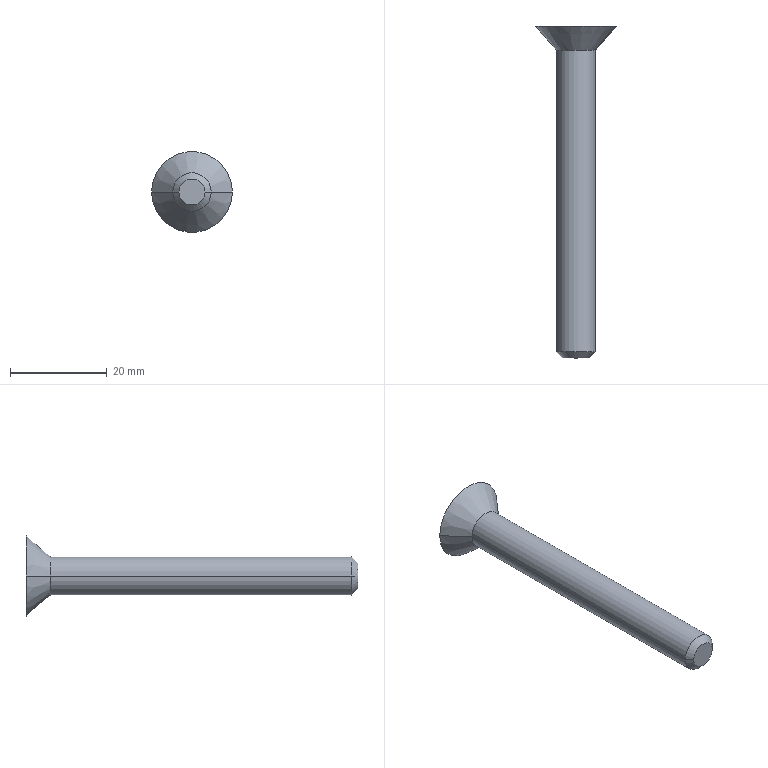Part | NX | features BREP 1 | 1 solid | 15 faces | box 16.681 x 68.529 x 16.681 mm | volume 3731 mm3 | plane 9 | cone 4 | cylinder 2 | commonest cylinder face diameters 7.938 x2
STEP:
#1=CARTESIAN_POINT('',(8.341,0.,0.));
#2=VERTEX_POINT('',#1);
#3=CARTESIAN_POINT('',(3.969,-5.029,0.));
#4=VERTEX_POINT('',#3);
#5=CARTESIAN_POINT('',(3.969,-5.029,0.));
#6=DIRECTION('',(0.6561,0.7547,0.));
#7=VECTOR('',#6,1000.);
#8=LINE('',#5,#7);
#9=EDGE_CURVE('',#2,#4,#8,.F.);
#10=ORIENTED_EDGE('',*,*,#9,.F.);
#11=CARTESIAN_POINT('',(-8.341,0.,0.));
#12=VERTEX_POINT('',#11);
#13=CARTESIAN_POINT('',(0.,0.,0.));
#14=DIRECTION('',(0.,-1.,0.));
#15=DIRECTION('',(1.,0.,0.));
#16=AXIS2_PLACEMENT_3D('',#13,#14,#15);
#17=CIRCLE('',#16,8.341);
#18=EDGE_CURVE('',#2,#12,#17,.T.);
#19=ORIENTED_EDGE('',*,*,#18,.T.);
#20=CARTESIAN_POINT('',(-3.969,-5.029,0.));
#21=VERTEX_POINT('',#20);
#22=CARTESIAN_POINT('',(-3.969,-5.029,0.));
#23=DIRECTION('',(-0.6561,0.7547,0.));
#24=VECTOR('',#23,1000.);
#25=LINE('',#22,#24);
#26=EDGE_CURVE('',#12,#21,#25,.F.);
#27=ORIENTED_EDGE('',*,*,#26,.T.);
#28=CARTESIAN_POINT('',(0.,-5.029,0.));
#29=DIRECTION('',(0.,-1.,0.));
#30=DIRECTION('',(1.,0.,0.));
#31=AXIS2_PLACEMENT_3D('',#28,#29,#30);
#32=CIRCLE('',#31,3.969);
#33=EDGE_CURVE('',#4,#21,#32,.T.);
#34=ORIENTED_EDGE('',*,*,#33,.F.);
#35=EDGE_LOOP('',(#10,#19,#27,#34));
#36=FACE_BOUND('',#35,.T.);
#37=CARTESIAN_POINT('',(0.,-2.515,0.));
#38=DIRECTION('',(0.,1.,0.));
#39=DIRECTION('',(1.,0.,0.));
#40=AXIS2_PLACEMENT_3D('',#37,#38,#39);
#41=CONICAL_SURFACE('',#40,6.155,0.7156);
#42=ADVANCED_FACE('',(#36),#41,.T.);
#43=CARTESIAN_POINT('',(-3.969,-67.259,0.));
#44=VERTEX_POINT('',#43);
#45=CARTESIAN_POINT('',(-3.969,-5.029,0.));
#46=DIRECTION('',(0.,-1.,0.));
#47=VECTOR('',#46,1000.);
#48=LINE('',#45,#47);
#49=EDGE_CURVE('',#21,#44,#48,.T.);
#50=ORIENTED_EDGE('',*,*,#49,.T.);
#51=CARTESIAN_POINT('',(3.969,-67.259,0.));
#52=VERTEX_POINT('',#51);
#53=CARTESIAN_POINT('',(0.,-67.259,0.));
#54=DIRECTION('',(0.,-1.,0.));
#55=DIRECTION('',(1.,0.,0.));
#56=AXIS2_PLACEMENT_3D('',#53,#54,#55);
#57=CIRCLE('',#56,3.969);
#58=EDGE_CURVE('',#52,#44,#57,.T.);
#59=ORIENTED_EDGE('',*,*,#58,.F.);
#60=CARTESIAN_POINT('',(3.969,-5.029,0.));
#61=DIRECTION('',(0.,-1.,0.));
#62=VECTOR('',#61,1000.);
#63=LINE('',#60,#62);
#64=EDGE_CURVE('',#4,#52,#63,.T.);
#65=ORIENTED_EDGE('',*,*,#64,.F.);
#66=ORIENTED_EDGE('',*,*,#33,.T.);
#67=EDGE_LOOP('',(#50,#59,#65,#66));
#68=FACE_BOUND('',#67,.T.);
#69=CARTESIAN_POINT('',(0.,-5.029,0.));
#70=DIRECTION('',(0.,-1.,0.));
#71=DIRECTION('',(1.,0.,0.));
#72=AXIS2_PLACEMENT_3D('',#69,#70,#71);
#73=CYLINDRICAL_SURFACE('',#72,3.969);
#74=ADVANCED_FACE('',(#68),#73,.T.);
#75=ORIENTED_EDGE('',*,*,#64,.T.);
#76=CARTESIAN_POINT('',(0.,-67.259,0.));
#77=DIRECTION('',(0.,-1.,0.));
#78=DIRECTION('',(-1.,0.,0.));
#79=AXIS2_PLACEMENT_3D('',#76,#77,#78);
#80=CIRCLE('',#79,3.969);
#81=EDGE_CURVE('',#44,#52,#80,.T.);
#82=ORIENTED_EDGE('',*,*,#81,.F.);
#83=ORIENTED_EDGE('',*,*,#49,.F.);
#84=CARTESIAN_POINT('',(0.,-5.029,0.));
#85=DIRECTION('',(0.,-1.,0.));
#86=DIRECTION('',(-1.,0.,0.));
#87=AXIS2_PLACEMENT_3D('',#84,#85,#86);
#88=CIRCLE('',#87,3.969);
#89=EDGE_CURVE('',#21,#4,#88,.T.);
#90=ORIENTED_EDGE('',*,*,#89,.T.);
#91=EDGE_LOOP('',(#75,#82,#83,#90));
#92=FACE_BOUND('',#91,.T.);
#93=CARTESIAN_POINT('',(0.,-5.029,0.));
#94=DIRECTION('',(0.,-1.,0.));
#95=DIRECTION('',(1.,0.,0.));
#96=AXIS2_PLACEMENT_3D('',#93,#94,#95);
#97=CYLINDRICAL_SURFACE('',#96,3.969);
#98=ADVANCED_FACE('',(#92),#97,.T.);
#99=ORIENTED_EDGE('',*,*,#26,.F.);
#100=CARTESIAN_POINT('',(0.,0.,0.));
#101=DIRECTION('',(0.,1.,0.));
#102=DIRECTION('',(1.,0.,0.));
#103=AXIS2_PLACEMENT_3D('',#100,#101,#102);
#104=CIRCLE('',#103,8.341);
#105=EDGE_CURVE('',#2,#12,#104,.T.);
#106=ORIENTED_EDGE('',*,*,#105,.F.);
#107=ORIENTED_EDGE('',*,*,#9,.T.);
#108=ORIENTED_EDGE('',*,*,#89,.F.);
#109=EDGE_LOOP('',(#99,#106,#107,#108));
#110=FACE_BOUND('',#109,.T.);
#111=CARTESIAN_POINT('',(0.,-2.515,0.));
#112=DIRECTION('',(0.,1.,0.));
#113=DIRECTION('',(1.,0.,0.));
#114=AXIS2_PLACEMENT_3D('',#111,#112,#113);
#115=CONICAL_SURFACE('',#114,6.155,0.7156);
#116=ADVANCED_FACE('',(#110),#115,.T.);
#117=ORIENTED_EDGE('',*,*,#18,.F.);
#118=ORIENTED_EDGE('',*,*,#105,.T.);
#119=EDGE_LOOP('',(#117,#118));
#120=FACE_BOUND('',#119,.T.);
#121=CARTESIAN_POINT('',(-1.984,0.,-1.146));
#122=VERTEX_POINT('',#121);
#123=CARTESIAN_POINT('',(-1.984,0.,1.146));
#124=VERTEX_POINT('',#123);
#125=CARTESIAN_POINT('',(-1.984,0.,-1.146));
#126=DIRECTION('',(0.,0.,1.));
#127=VECTOR('',#126,1000.);
#128=LINE('',#125,#127);
#129=EDGE_CURVE('',#122,#124,#128,.T.);
#130=ORIENTED_EDGE('',*,*,#129,.F.);
#131=CARTESIAN_POINT('',(0.,0.,-2.291));
#132=VERTEX_POINT('',#131);
#133=CARTESIAN_POINT('',(0.,0.,-2.291));
#134=DIRECTION('',(-0.866,0.,0.5));
#135=VECTOR('',#134,1000.);
#136=LINE('',#133,#135);
#137=EDGE_CURVE('',#132,#122,#136,.T.);
#138=ORIENTED_EDGE('',*,*,#137,.F.);
#139=CARTESIAN_POINT('',(1.984,0.,-1.146));
#140=VERTEX_POINT('',#139);
#141=CARTESIAN_POINT('',(1.984,0.,-1.146));
#142=DIRECTION('',(-0.866,0.,-0.5));
#143=VECTOR('',#142,1000.);
#144=LINE('',#141,#143);
#145=EDGE_CURVE('',#140,#132,#144,.T.);
#146=ORIENTED_EDGE('',*,*,#145,.F.);
#147=CARTESIAN_POINT('',(1.984,0.,1.146));
#148=VERTEX_POINT('',#147);
#149=CARTESIAN_POINT('',(1.984,0.,1.146));
#150=DIRECTION('',(0.,0.,-1.));
#151=VECTOR('',#150,1000.);
#152=LINE('',#149,#151);
#153=EDGE_CURVE('',#148,#140,#152,.T.);
#154=ORIENTED_EDGE('',*,*,#153,.F.);
#155=CARTESIAN_POINT('',(0.,0.,2.291));
#156=VERTEX_POINT('',#155);
#157=CARTESIAN_POINT('',(0.,0.,2.291));
#158=DIRECTION('',(0.866,0.,-0.5));
#159=VECTOR('',#158,1000.);
#160=LINE('',#157,#159);
#161=EDGE_CURVE('',#156,#148,#160,.T.);
#162=ORIENTED_EDGE('',*,*,#161,.F.);
#163=CARTESIAN_POINT('',(-1.984,0.,1.146));
#164=DIRECTION('',(0.866,0.,0.5));
#165=VECTOR('',#164,1000.);
#166=LINE('',#163,#165);
#167=EDGE_CURVE('',#124,#156,#166,.T.);
#168=ORIENTED_EDGE('',*,*,#167,.F.);
#169=EDGE_LOOP('',(#130,#138,#146,#154,#162,#168));
#170=FACE_BOUND('',#169,.T.);
#171=CARTESIAN_POINT('',(0.,0.,0.));
#172=DIRECTION('',(0.,-1.,0.));
#173=DIRECTION('',(0.,0.,-1.));
#174=AXIS2_PLACEMENT_3D('',#171,#172,#173);
#175=PLANE('',#174);
#176=ADVANCED_FACE('',(#120,#170),#175,.F.);
#177=CARTESIAN_POINT('',(0.,-1.27,2.291));
#178=VERTEX_POINT('',#177);
#179=CARTESIAN_POINT('',(0.,0.,2.291));
#180=DIRECTION('',(0.,-1.,0.));
#181=VECTOR('',#180,1000.);
#182=LINE('',#179,#181);
#183=EDGE_CURVE('',#156,#178,#182,.T.);
#184=ORIENTED_EDGE('',*,*,#183,.T.);
#185=CARTESIAN_POINT('',(-1.984,-1.27,1.146));
#186=VERTEX_POINT('',#185);
#187=CARTESIAN_POINT('',(-1.984,-1.27,1.146));
#188=DIRECTION('',(0.866,0.,0.5));
#189=VECTOR('',#188,1000.);
#190=LINE('',#187,#189);
#191=EDGE_CURVE('',#186,#178,#190,.T.);
#192=ORIENTED_EDGE('',*,*,#191,.F.);
#193=CARTESIAN_POINT('',(-1.984,0.,1.146));
#194=DIRECTION('',(0.,-1.,0.));
#195=VECTOR('',#194,1000.);
#196=LINE('',#193,#195);
#197=EDGE_CURVE('',#124,#186,#196,.T.);
#198=ORIENTED_EDGE('',*,*,#197,.F.);
#199=ORIENTED_EDGE('',*,*,#167,.T.);
#200=EDGE_LOOP('',(#184,#192,#198,#199));
#201=FACE_BOUND('',#200,.T.);
#202=CARTESIAN_POINT('',(-1.984,0.,1.146));
#203=DIRECTION('',(-0.5,0.,0.866));
#204=DIRECTION('',(0.,1.,0.));
#205=AXIS2_PLACEMENT_3D('',#202,#203,#204);
#206=PLANE('',#205);
#207=ADVANCED_FACE('',(#201),#206,.F.);
#208=ORIENTED_EDGE('',*,*,#197,.T.);
#209=CARTESIAN_POINT('',(-1.984,-1.27,-1.146));
#210=VERTEX_POINT('',#209);
#211=CARTESIAN_POINT('',(-1.984,-1.27,-1.146));
#212=DIRECTION('',(0.,0.,1.));
#213=VECTOR('',#212,1000.);
#214=LINE('',#211,#213);
#215=EDGE_CURVE('',#210,#186,#214,.T.);
#216=ORIENTED_EDGE('',*,*,#215,.F.);
#217=CARTESIAN_POINT('',(-1.984,0.,-1.146));
#218=DIRECTION('',(0.,-1.,0.));
#219=VECTOR('',#218,1000.);
#220=LINE('',#217,#219);
#221=EDGE_CURVE('',#122,#210,#220,.T.);
#222=ORIENTED_EDGE('',*,*,#221,.F.);
#223=ORIENTED_EDGE('',*,*,#129,.T.);
#224=EDGE_LOOP('',(#208,#216,#222,#223));
#225=FACE_BOUND('',#224,.T.);
#226=CARTESIAN_POINT('',(-1.984,0.,-1.146));
#227=DIRECTION('',(-1.,0.,0.));
#228=DIRECTION('',(0.,0.,1.));
#229=AXIS2_PLACEMENT_3D('',#226,#227,#228);
#230=PLANE('',#229);
#231=ADVANCED_FACE('',(#225),#230,.F.);
#232=ORIENTED_EDGE('',*,*,#221,.T.);
#233=CARTESIAN_POINT('',(0.,-1.27,-2.291));
#234=VERTEX_POINT('',#233);
#235=CARTESIAN_POINT('',(0.,-1.27,-2.291));
#236=DIRECTION('',(-0.866,0.,0.5));
#237=VECTOR('',#236,1000.);
#238=LINE('',#235,#237);
#239=EDGE_CURVE('',#234,#210,#238,.T.);
#240=ORIENTED_EDGE('',*,*,#239,.F.);
#241=CARTESIAN_POINT('',(0.,0.,-2.291));
#242=DIRECTION('',(0.,-1.,0.));
#243=VECTOR('',#242,1000.);
#244=LINE('',#241,#243);
#245=EDGE_CURVE('',#132,#234,#244,.T.);
#246=ORIENTED_EDGE('',*,*,#245,.F.);
#247=ORIENTED_EDGE('',*,*,#137,.T.);
#248=EDGE_LOOP('',(#232,#240,#246,#247));
#249=FACE_BOUND('',#248,.T.);
#250=CARTESIAN_POINT('',(0.,0.,-2.291));
#251=DIRECTION('',(-0.5,0.,-0.866));
#252=DIRECTION('',(-0.866,0.,0.5));
#253=AXIS2_PLACEMENT_3D('',#250,#251,#252);
#254=PLANE('',#253);
#255=ADVANCED_FACE('',(#249),#254,.F.);
#256=ORIENTED_EDGE('',*,*,#245,.T.);
#257=CARTESIAN_POINT('',(1.984,-1.27,-1.146));
#258=VERTEX_POINT('',#257);
#259=CARTESIAN_POINT('',(1.984,-1.27,-1.146));
#260=DIRECTION('',(-0.866,0.,-0.5));
#261=VECTOR('',#260,1000.);
#262=LINE('',#259,#261);
#263=EDGE_CURVE('',#258,#234,#262,.T.);
#264=ORIENTED_EDGE('',*,*,#263,.F.);
#265=CARTESIAN_POINT('',(1.984,0.,-1.146));
#266=DIRECTION('',(0.,-1.,0.));
#267=VECTOR('',#266,1000.);
#268=LINE('',#265,#267);
#269=EDGE_CURVE('',#140,#258,#268,.T.);
#270=ORIENTED_EDGE('',*,*,#269,.F.);
#271=ORIENTED_EDGE('',*,*,#145,.T.);
#272=EDGE_LOOP('',(#256,#264,#270,#271));
#273=FACE_BOUND('',#272,.T.);
#274=CARTESIAN_POINT('',(1.984,0.,-1.146));
#275=DIRECTION('',(0.5,0.,-0.866));
#276=DIRECTION('',(0.,-1.,0.));
#277=AXIS2_PLACEMENT_3D('',#274,#275,#276);
#278=PLANE('',#277);
#279=ADVANCED_FACE('',(#273),#278,.F.);
#280=ORIENTED_EDGE('',*,*,#269,.T.);
#281=CARTESIAN_POINT('',(1.984,-1.27,1.146));
#282=VERTEX_POINT('',#281);
#283=CARTESIAN_POINT('',(1.984,-1.27,1.146));
#284=DIRECTION('',(0.,0.,-1.));
#285=VECTOR('',#284,1000.);
#286=LINE('',#283,#285);
#287=EDGE_CURVE('',#282,#258,#286,.T.);
#288=ORIENTED_EDGE('',*,*,#287,.F.);
#289=CARTESIAN_POINT('',(1.984,0.,1.146));
#290=DIRECTION('',(0.,-1.,0.));
#291=VECTOR('',#290,1000.);
#292=LINE('',#289,#291);
#293=EDGE_CURVE('',#148,#282,#292,.T.);
#294=ORIENTED_EDGE('',*,*,#293,.F.);
#295=ORIENTED_EDGE('',*,*,#153,.T.);
#296=EDGE_LOOP('',(#280,#288,#294,#295));
#297=FACE_BOUND('',#296,.T.);
#298=CARTESIAN_POINT('',(1.984,0.,1.146));
#299=DIRECTION('',(1.,0.,0.));
#300=DIRECTION('',(0.,1.,0.));
#301=AXIS2_PLACEMENT_3D('',#298,#299,#300);
#302=PLANE('',#301);
#303=ADVANCED_FACE('',(#297),#302,.F.);
#304=ORIENTED_EDGE('',*,*,#293,.T.);
#305=CARTESIAN_POINT('',(0.,-1.27,2.291));
#306=DIRECTION('',(0.866,0.,-0.5));
#307=VECTOR('',#306,1000.);
#308=LINE('',#305,#307);
#309=EDGE_CURVE('',#178,#282,#308,.T.);
#310=ORIENTED_EDGE('',*,*,#309,.F.);
#311=ORIENTED_EDGE('',*,*,#183,.F.);
#312=ORIENTED_EDGE('',*,*,#161,.T.);
#313=EDGE_LOOP('',(#304,#310,#311,#312));
#314=FACE_BOUND('',#313,.T.);
#315=CARTESIAN_POINT('',(0.,0.,2.291));
#316=DIRECTION('',(0.5,0.,0.866));
#317=DIRECTION('',(0.,-1.,0.));
#318=AXIS2_PLACEMENT_3D('',#315,#316,#317);
#319=PLANE('',#318);
#320=ADVANCED_FACE('',(#314),#319,.F.);
#321=ORIENTED_EDGE('',*,*,#309,.T.);
#322=ORIENTED_EDGE('',*,*,#287,.T.);
#323=ORIENTED_EDGE('',*,*,#263,.T.);
#324=ORIENTED_EDGE('',*,*,#239,.T.);
#325=ORIENTED_EDGE('',*,*,#215,.T.);
#326=ORIENTED_EDGE('',*,*,#191,.T.);
#327=EDGE_LOOP('',(#321,#322,#323,#324,#325,#326));
#328=FACE_BOUND('',#327,.T.);
#329=CARTESIAN_POINT('',(0.,-1.27,0.));
#330=DIRECTION('',(0.,1.,0.));
#331=DIRECTION('',(1.,0.,0.));
#332=AXIS2_PLACEMENT_3D('',#329,#330,#331);
#333=PLANE('',#332);
#334=ADVANCED_FACE('',(#328),#333,.T.);
#335=CARTESIAN_POINT('',(-2.699,-68.529,0.));
#336=VERTEX_POINT('',#335);
#337=CARTESIAN_POINT('',(-2.699,-68.529,0.));
#338=DIRECTION('',(-0.7071,0.7071,0.));
#339=VECTOR('',#338,1000.);
#340=LINE('',#337,#339);
#341=EDGE_CURVE('',#336,#44,#340,.T.);
#342=ORIENTED_EDGE('',*,*,#341,.T.);
#343=ORIENTED_EDGE('',*,*,#81,.T.);
#344=CARTESIAN_POINT('',(2.699,-68.529,0.));
#345=VERTEX_POINT('',#344);
#346=CARTESIAN_POINT('',(2.699,-68.529,0.));
#347=DIRECTION('',(0.7071,0.7071,0.));
#348=VECTOR('',#347,1000.);
#349=LINE('',#346,#348);
#350=EDGE_CURVE('',#345,#52,#349,.T.);
#351=ORIENTED_EDGE('',*,*,#350,.F.);
#352=CARTESIAN_POINT('',(0.,-68.529,0.));
#353=DIRECTION('',(0.,-1.,0.));
#354=DIRECTION('',(-1.,0.,0.));
#355=AXIS2_PLACEMENT_3D('',#352,#353,#354);
#356=CIRCLE('',#355,2.699);
#357=EDGE_CURVE('',#336,#345,#356,.T.);
#358=ORIENTED_EDGE('',*,*,#357,.F.);
#359=EDGE_LOOP('',(#342,#343,#351,#358));
#360=FACE_BOUND('',#359,.T.);
#361=CARTESIAN_POINT('',(0.,-67.894,0.));
#362=DIRECTION('',(0.,1.,0.));
#363=DIRECTION('',(-1.,0.,0.));
#364=AXIS2_PLACEMENT_3D('',#361,#362,#363);
#365=CONICAL_SURFACE('',#364,3.334,0.7854);
#366=ADVANCED_FACE('',(#360),#365,.T.);
#367=ORIENTED_EDGE('',*,*,#357,.T.);
#368=CARTESIAN_POINT('',(0.,-68.529,0.));
#369=DIRECTION('',(0.,-1.,0.));
#370=DIRECTION('',(1.,0.,0.));
#371=AXIS2_PLACEMENT_3D('',#368,#369,#370);
#372=CIRCLE('',#371,2.699);
#373=EDGE_CURVE('',#345,#336,#372,.T.);
#374=ORIENTED_EDGE('',*,*,#373,.T.);
#375=EDGE_LOOP('',(#367,#374));
#376=FACE_BOUND('',#375,.T.);
#377=CARTESIAN_POINT('',(0.,-68.529,0.));
#378=DIRECTION('',(0.,-1.,0.));
#379=DIRECTION('',(0.,0.,-1.));
#380=AXIS2_PLACEMENT_3D('',#377,#378,#379);
#381=PLANE('',#380);
#382=ADVANCED_FACE('',(#376),#381,.T.);
#383=ORIENTED_EDGE('',*,*,#350,.T.);
#384=ORIENTED_EDGE('',*,*,#58,.T.);
#385=ORIENTED_EDGE('',*,*,#341,.F.);
#386=ORIENTED_EDGE('',*,*,#373,.F.);
#387=EDGE_LOOP('',(#383,#384,#385,#386));
#388=FACE_BOUND('',#387,.T.);
#389=CARTESIAN_POINT('',(0.,-67.894,0.));
#390=DIRECTION('',(0.,1.,0.));
#391=DIRECTION('',(-1.,0.,0.));
#392=AXIS2_PLACEMENT_3D('',#389,#390,#391);
#393=CONICAL_SURFACE('',#392,3.334,0.7854);
#394=ADVANCED_FACE('',(#388),#393,.T.);
#395=CLOSED_SHELL('',(#42,#74,#98,#116,#176,#207,#231,#255,#279,#303,#320,#334,#366,#382,#394));
#396=MANIFOLD_SOLID_BREP('',#395);
#397=(LENGTH_UNIT()NAMED_UNIT(*)SI_UNIT(.MILLI.,.METRE.));
#398=UNCERTAINTY_MEASURE_WITH_UNIT(LENGTH_MEASURE(0.00001),#397,'','');
#399=(NAMED_UNIT(*)PLANE_ANGLE_UNIT()SI_UNIT($,.RADIAN.));
#400=(NAMED_UNIT(*)SI_UNIT($,.STERADIAN.)SOLID_ANGLE_UNIT());
#401=(GEOMETRIC_REPRESENTATION_CONTEXT(3)GLOBAL_UNCERTAINTY_ASSIGNED_CONTEXT((#398))GLOBAL_UNIT_ASSIGNED_CONTEXT((#397,#399,#400))REPRESENTATION_CONTEXT('',''));
#402=ADVANCED_BREP_SHAPE_REPRESENTATION('',(#396),#401);